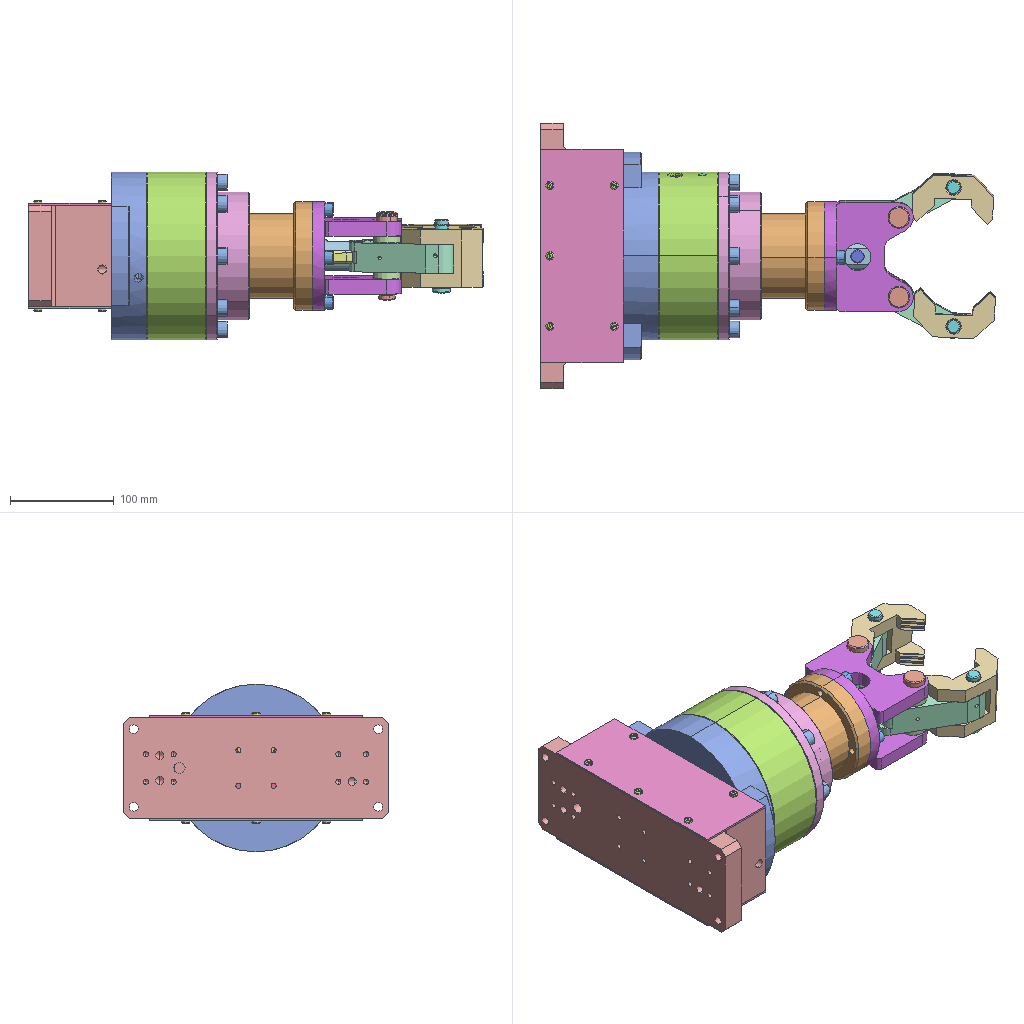Assembly | SolidWorks | 43 different items | 84 placed | box 439 x 256 x 162 mm
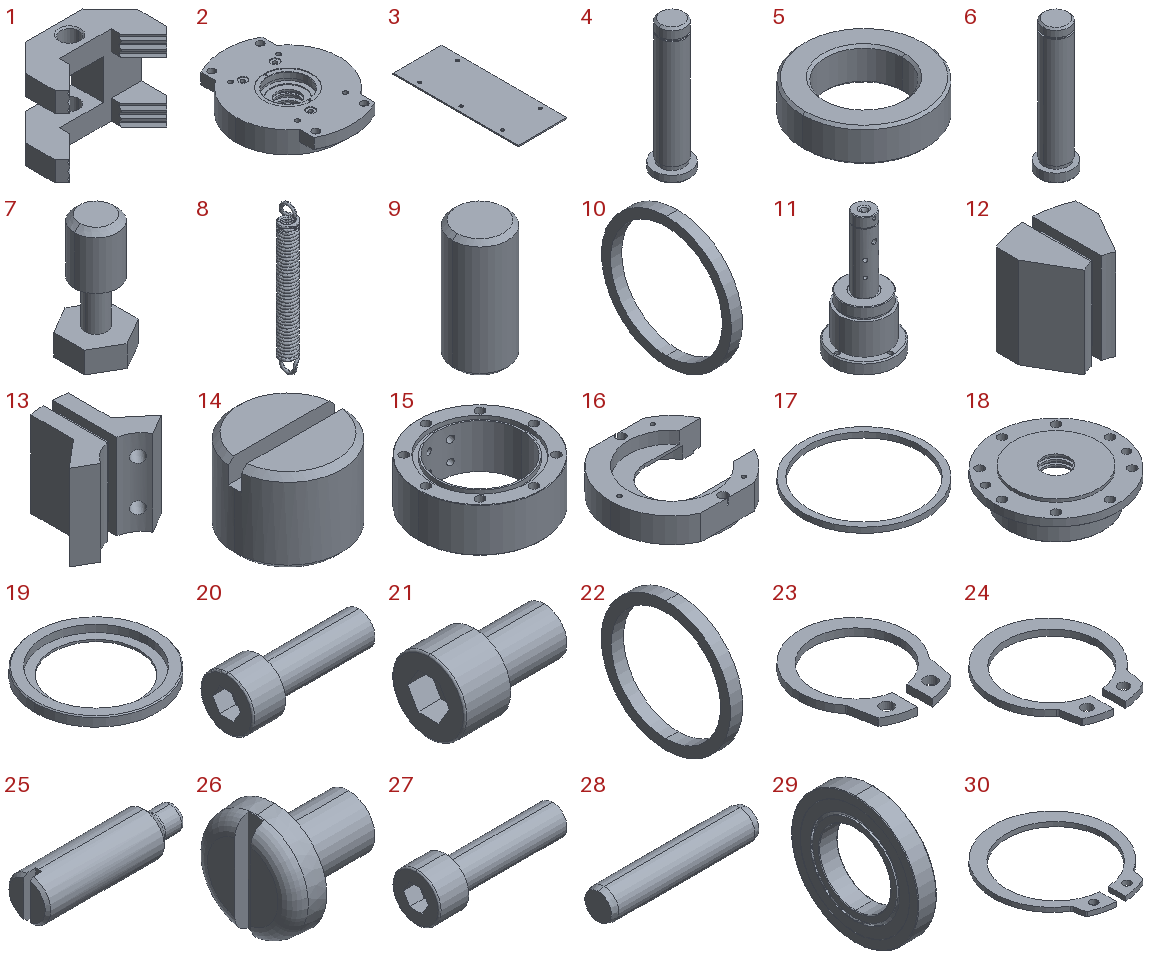Parts list (item | quantity | size | volume | features):
1 | x2 | 78 x 44.997 x 56 mm | 64045 mm3 | features ICE 3, MirrorPattern 2, Chamfer 1, Extrusion 1
2 | x1 | 162 x 200 x 38 mm | 697983 mm3 | features ICE 13, HoleWzd 9, Chamfer 2, 3DProfileFeature 1, CirPattern 1, Extrusion 1, MirrorPattern 1
3 | x2 | 80 x 206 x 2 mm | 32764 mm3 | features Extrusion 1, HoleWzd 1
4 | x2 | 18 x 18 x 66 mm | 9140 mm3 | features ICE 4, Chamfer 1, Extrusion 1
5 | x2 | 26 x 26 x 7 mm | 2241 mm3 | features Chamfer 1, Extrusion 1
6 | x2 | 21 x 21 x 82 mm | 17223 mm3 | features ICE 4, Chamfer 1, Extrusion 1
7 | x1 | 5 x 5.774 x 11 mm | 117.26 mm3 | features ICE 2, Chamfer 1, Extrusion 1
8 | x1 | 5.989 x 6.003 x 53 mm | 518.141 mm3 | features RefCurve 2, CompositeCurve 1, Helix 1, Sweep 1
9 | x1 | 13 x 13 x 28 mm | 3662 mm3 | features 3DProfileFeature 1, Chamfer 1, Extrusion 1, HoleWzd 1
10 | x4 | 3.5 x 40.6 x 40.6 mm | 1164 mm3 | features Extrusion 1
11 | x1 | 105 x 105 x 207 mm | 339830 mm3 | features ICE 8, HoleWzd 5, 3DProfileFeature 4, RevCut 3, Chamfer 2, CirPattern 1, Extrusion 1
12 | x1 | 44 x 39.776 x 50 mm | 60767 mm3 | features 3DProfileFeature 2, HoleWzd 2, Extrusion 1, ICE 1
13 | x1 | 53.823 x 46.181 x 50 mm | 52873 mm3 | features 3DProfileFeature 2, HoleWzd 2, Extrusion 1, ICE 1
14 | x1 | 9.73 x 9.73 x 7.5 mm | 527.297 mm3 | features Chamfer 1, Extrusion 1, ICE 1
15 | x1 | 162 x 162 x 58 mm | 564661 mm3 | features HoleWzd 5, 3DProfileFeature 4, Chamfer 2, ICE 2, CirPattern 1, Extrusion 1, MirrorPattern 1
16 | x1 | 77.837 x 73.95 x 18 mm | 34057 mm3 | features ICE 5, 3DProfileFeature 2, HoleWzd 2, CirPattern 1, Extrusion 1
17 | x2 | 127 x 127 x 5.5 mm | 13534 mm3 | features Extrusion 1
18 | x1 | 162 x 162 x 45 mm | 267421 mm3 | features ICE 12, Chamfer 2, HoleWzd 2, CirPattern 1, Extrusion 1
19 | x1 | 120 x 120 x 9 mm | 34518 mm3 | features Chamfer 1, CirPattern 1, Extrusion 1, HoleWzd 1, ICE 1
20 | x4 | 33 x 13 x 13 mm | 2188 mm3 | features BlendCut 1, Cut 1, Fillet 1, LPattern 1, RevCut 1, Revolution 1
21 | x4 | 26 x 16 x 16 mm | 2981 mm3 | features BlendCut 1, Cut 1, Fillet 1, LPattern 1, RevCut 1, Revolution 1
22 | x2 | 6.2 x 65 x 65 mm | 5843 mm3 | features Extrusion 1
23 | x2 | 14.7 x 17.116 x 1 mm | 75.123 mm3 | features Extrusion 1
24 | x2 | 18.2 x 20.685 x 1 mm | 106.213 mm3 | features Extrusion 1
25 | x1 | 14 x 4 x 4 mm | 151.43 mm3 | features Cut 1, Fillet 1, Revolution 1
26 | x10 | 8.4 x 8 x 8 mm | 170.552 mm3 | features Fillet 2, ICE 1, LPattern 1, RevCut 1, Revolution 1
27 | x2 | 38 x 13 x 13 mm | 2439 mm3 | features BlendCut 1, Cut 1, Fillet 1, LPattern 1, RevCut 1, Revolution 1
28 | x2 | 40 x 8 x 8 mm | 1994 mm3 | features Revolution 1
29 | x1 | 9 x 62 x 62 mm | 14273 mm3 | features Revolution 5, CirPattern 2, RefAxis 1, RevCut 1
30 | x1 | 39 x 42.278 x 1.5 mm | 631.207 mm3 | features Extrusion 1
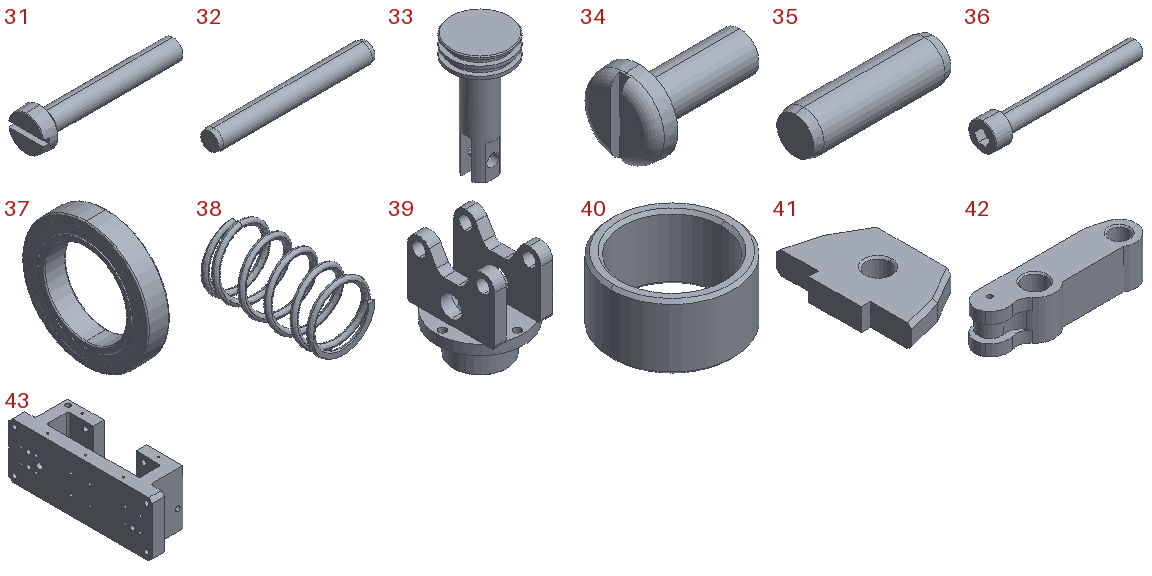31 | x2 | 22 x 5.5 x 5.5 mm | 181.48 mm3 | features Cut 1, LPattern 1, RevCut 1, Revolution 1
32 | x2 | 80 x 10 x 10 mm | 6251 mm3 | features Revolution 1
33 | x1 | 65 x 65 x 132 mm | 129865 mm3 | features ICE 9, Chamfer 2, 3DProfileFeature 1, Extrusion 1, Fillet 1, HoleWzd 1
34 | x2 | 19.6 x 12 x 12 mm | 779.516 mm3 | features Fillet 2, ICE 1, LPattern 1, RevCut 1, Revolution 1
35 | x2 | 20 x 6 x 6 mm | 558.473 mm3 | features Revolution 1
36 | x8 | 90 x 16 x 16 mm | 8007 mm3 | features BlendCut 1, Cut 1, Fillet 1, LPattern 1, RevCut 1, Revolution 1
37 | x1 | 20 x 115 x 115 mm | 89523 mm3 | features Revolution 5, CirPattern 2, RefAxis 1, RevCut 1
38 | x1 | 52.5 x 90 x 52.5 mm | 16226 mm3 | features Sweep 3, ICE 1
39 | x1 | 105 x 105 x 121 mm | 288866 mm3 | features ICE 4, Chamfer 1, CirPattern 1, Extrusion 1, Fillet 1, HoleWzd 1, MirrorPattern 1
40 | x1 | 40 x 40 x 21 mm | 9274 mm3 | features Chamfer 1, Extrusion 1
41 | x1 | 41 x 72 x 12 mm | 25554 mm3 | features Chamfer 2, Extrusion 1
42 | x2 | 109.566 x 29 x 28 mm | 60118 mm3 | features ICE 3, MirrorPattern 2, 3DProfileFeature 1, Chamfer 1, Extrusion 1, HoleWzd 1
43 | x1 | 80 x 256 x 98 mm | 906653 mm3 | features HoleWzd 16, MirrorPattern 3, 3DProfileFeature 2, Chamfer 1, CirPattern 1, Extrusion 1, Fillet 1, ICE 1
Mates (type | each side: item.copy, entity, surface, feature):
Coincident | 43.1 face plane Boss-Extrude2 | 2.1 face plane Boss-Extrude1
Concentric | 43.1 face cylinder M10 Tapped Hole2 | 2.1 face cylinder Mirror1
Concentric | 43.1 face cylinder M10 Tapped Hole2 | 2.1 face cylinder CBORE for M1.6 Hex Head Bolt2
Coincident | 2.1 face plane Boss-Extrude2 | 15.1 face plane Boss-Extrude1
Concentric | 2.1 face cylinder M10 Tapped Hole2 | 15.1 face cylinder Ø5.0mm Blind Dowel Hole1
Concentric | 2.1 face cylinder CirPattern1 | 15.1 face cylinder CirPattern1
Coincident | 15.1 face plane Boss-Extrude1 | 18.1 face plane Boss-Extrude1
Concentric | 15.1 face cylinder Ø5.0mm Blind Dowel Hole1 | 18.1 face cylinder CirPattern1
Concentric | 15.1 face cylinder CirPattern1 | 18.1 face cylinder CirPattern1
Parallel | 18.1 face plane Cut-Extrude6 | 19.1 face plane Boss-Extrude1
Coincident | 18.1 face plane Boss-Extrude3 | 19.1 face plane Boss-Extrude1
Concentric | 18.1 edge | 19.1 edge
Parallel | 19.1 plane | assembly plane
Concentric | 15.1 face cylinder Ø8.0mm Blind Dowel Hole1 | 12.1 face cylinder Ø8.0mm Blind Dowel Hole1
Coincident | 18.1 face plane Boss-Extrude2 | 12.1 face plane Boss-Extrude1
Concentric | 15.1 face cylinder Ø8.0mm Blind Dowel Hole2 | 12.1 face cylinder Ø8.0mm Blind Dowel Hole1
Concentric | 2.1 face cylinder Cut-Extrude11 | 11.1 face cone Cut-Revolve2
Parallel | 13.1 plane | assembly plane
Concentric | 11.1 face cylinder Ø6.0mm Blind Dowel Hole1 | 13.1 face cylinder Ø6.0mm Blind Dowel Hole2
Concentric | 11.1 face cylinder Ø6.0mm Blind Dowel Hole1 | 13.1 face cylinder Ø6.0mm Blind Dowel Hole1
Coincident | 18.1 face plane Boss-Extrude2 | 13.1 face plane Boss-Extrude1
Concentric | 11.1 face cylinder Cut-Revolve2 | 16.1 face cylinder Cut-Extrude5
Parallel | 43.1 face plane Boss-Extrude2 | 16.1 face plane Cut-Extrude1
Coincident | 2.1 face plane Cut-Extrude1 | 16.1 face plane Boss-Extrude2
Concentric | 11.1 edge | 33.1 edge
Concentric | 33.1 face cylinder Cut-Extrude3 | 41.1 face cylinder Boss-Extrude1
Coincident | 33.1 face plane Cut-Extrude1 | 41.1 face plane Boss-Extrude1
Coincident | 11.1 face plane Boss-Extrude1 | 39.1 face plane Boss-Extrude2
Concentric | 11.1 face cylinder M8 Tapped Hole1 | 39.1 face cylinder CirPattern1
Concentric | 11.1 face cylinder CirPattern1 | 39.1 face cylinder Ø5.0mm Blind Dowel Hole1
LimitDistanceDim | 33.1 face plane Boss-Extrude5 | 11.1 face plane Cut-Extrude2
Parallel | 33.1 face plane Cut-Extrude1 | 41.1 face plane Boss-Extrude1
Concentric | 39.1 face cylinder Mirror1 | 42.1 face cylinder Boss-Extrude1
Concentric | 39.1 face cylinder Mirror1 | 42.2 face cylinder Boss-Extrude1
Width | 39.1 face plane Boss-Extrude3 | 39.1 face plane Mirror1 | 42.1 face plane Mirror1 | 42.1 face plane Boss-Extrude2
Concentric | 39.1 face cylinder Boss-Extrude3 | 6.1 face cylinder Boss-Extrude3
Coincident | 39.1 face plane Mirror1 | 6.1 face plane Boss-Extrude1
Width | 39.1 face plane Mirror1 | 39.1 face plane Boss-Extrude3 | 42.2 face plane Mirror1 | 42.2 face plane Boss-Extrude2
Concentric | 39.1 face cylinder Mirror1 | 6.2 face cylinder Boss-Extrude3
Coincident | 39.1 face plane Mirror1 | 6.2 edge
Parallel | 41.1 face plane Boss-Extrude1 | 39.1 face plane Boss-Extrude3
Concentric | 33.1 face cylinder Cut-Extrude3 | 9.1 face cylinder Boss-Extrude1
Width | 9.1 face plane Boss-Extrude1 | 9.1 face plane Boss-Extrude1 | 33.1 face plane Cut-Extrude2 | 33.1 face plane Cut-Extrude2
Concentric | 33.1 face cylinder M4 Tapped Hole1 | 9.1 face cylinder Ø2.5mm Blind Dowel Hole1
Concentric | 6.2 face cylinder Boss-Extrude3 | 5.1 face cylinder Boss-Extrude1
Coincident | 42.2 face plane Boss-Extrude2 | 5.1 face plane Boss-Extrude1
Concentric | 6.2 face cylinder Boss-Extrude3 | 5.2 face cylinder Boss-Extrude1
Coincident | 39.1 face plane Mirror1 | 5.2 face plane Boss-Extrude1
Concentric | 43.1 face cylinder M4 Tapped Hole1 | 3.1 face cylinder Ø5.0mm Blind Dowel Hole1 | 2 times
Coincident | 43.1 face plane Boss-Extrude2 | 3.1 face plane Boss-Extrude1
Concentric | 43.1 face cylinder Mirror1 | 3.2 face cylinder Ø5.0mm Blind Dowel Hole1 | 2 times
Coincident | 43.1 face plane Boss-Extrude2 | 3.2 face plane Boss-Extrude1
Concentric | 42.2 face cylinder Boss-Extrude1 | 1.1 face cylinder Boss-Extrude1
Width | 1.1 face plane Boss-Extrude1 | 1.1 face plane Boss-Extrude1 | 42.2 face plane Boss-Extrude2 | 42.2 face plane Mirror1
Concentric | 4.1 face cylinder Boss-Extrude3 | 1.1 face cylinder Boss-Extrude1
Coincident | 1.1 face plane Boss-Extrude1 | 4.1 face plane Boss-Extrude5
Concentric | 42.1 face cylinder Boss-Extrude1 | 1.2 face cylinder Boss-Extrude1
Width | 1.2 face plane Boss-Extrude1 | 1.2 face plane Boss-Extrude1 | 42.1 face plane Boss-Extrude2 | 42.1 face plane Mirror1
Concentric | 1.2 face cylinder Boss-Extrude1 | 4.2 face cylinder Boss-Extrude3
Coincident | 1.2 face plane Boss-Extrude1 | 4.2 face plane Boss-Extrude5
Tangent | 41.1 face plane Boss-Extrude1 | 42.2 face cylinder Boss-Extrude1
Tangent | 41.1 face plane Boss-Extrude1 | 42.1 face cylinder Boss-Extrude1
Concentric | 11.1 face cylinder Cut-Revolve1 | 17.1 face cylinder Boss-Extrude1
Coincident | 2.1 face plane Boss-Extrude2 | 17.1 face plane Boss-Extrude1
Concentric | 11.1 face cylinder Cut-Revolve1 | 17.2 face cylinder Boss-Extrude1
Coincident | 18.1 face plane Boss-Extrude1 | 17.2 edge
Concentric | 11.1 face cylinder Cut-Extrude1 | 22.1 face cylinder Boss-Extrude1
Concentric | 11.1 face cylinder Cut-Extrude1 | 22.2 edge
Coincident | 33.1 face plane Boss-Extrude5 | 22.2 face plane Boss-Extrude1
Coincident | 33.1 face plane Boss-Extrude3 | 22.1 face plane Boss-Extrude1
Concentric | 11.1 face cylinder Cut-Revolve1 | 10.1 face cylinder Boss-Extrude1
Coincident | 18.1 face plane Cut-Extrude4 | 10.1 face plane Boss-Extrude1
Concentric | 11.1 face cylinder Cut-Revolve1 | 10.2 face cylinder Boss-Extrude1
Coincident | 18.1 face plane Cut-Extrude2 | 10.2 face plane Boss-Extrude1
Concentric | 11.1 face cylinder Cut-Revolve1 | 10.3 face cylinder Boss-Extrude1
Coincident | 2.1 face plane Cut-Extrude3 | 10.3 face plane Boss-Extrude1
Concentric | 11.1 face cylinder Cut-Revolve1 | 10.4 face cylinder Boss-Extrude1
Coincident | 2.1 face plane Cut-Extrude7 | 10.4 face plane Boss-Extrude1
Concentric | 18.1 face cylinder CirPattern1 | 36.1 face cylinder Base-Revolve
Coincident | 18.1 face plane Boss-Extrude1 | 36.1 face plane Base-Revolve
Concentric | 18.1 face cylinder CirPattern1 | 36.2 face cylinder Base-Revolve
Coincident | 18.1 face plane Boss-Extrude1 | 36.2 face plane Base-Revolve
Concentric | 18.1 face cylinder CirPattern1 | 36.3 face cylinder Base-Revolve
Coincident | 18.1 face plane Boss-Extrude1 | 36.3 face plane Base-Revolve
Concentric | 18.1 face cylinder Ø1.0mm Blind Dowel Hole1 | 36.4 face cylinder Base-Revolve
Coincident | 18.1 face plane Boss-Extrude1 | 36.4 edge
Concentric | 18.1 face cylinder CirPattern1 | 36.5 face cylinder Base-Revolve
Coincident | 18.1 face plane Boss-Extrude1 | 36.5 face plane Base-Revolve
Concentric | 18.1 face cylinder CirPattern1 | 36.6 face cylinder Base-Revolve
Coincident | 18.1 face plane Boss-Extrude1 | 36.6 face plane Base-Revolve
Concentric | 18.1 face cylinder CirPattern1 | 36.7 face cylinder Base-Revolve
Coincident | 18.1 face plane Boss-Extrude1 | 36.7 face plane Base-Revolve
Concentric | 18.1 face cylinder CirPattern1 | 36.8 face cylinder Base-Revolve
Coincident | 18.1 face plane Boss-Extrude1 | 36.8 edge
Concentric | 3.1 face cylinder Ø5.0mm Blind Dowel Hole1 | 26.1 face cylinder Base-Revolve
Coincident | 3.1 face plane Boss-Extrude1 | 26.1 face plane Base-Revolve
Concentric | 3.1 face cylinder Ø5.0mm Blind Dowel Hole1 | 26.2 face cylinder Base-Revolve
Coincident | 3.1 face plane Boss-Extrude1 | 26.2 face plane Base-Revolve
Concentric | 3.1 face cylinder Ø5.0mm Blind Dowel Hole1 | 26.3 face cylinder Base-Revolve
Coincident | 3.1 face plane Boss-Extrude1 | 26.3 face plane Base-Revolve
Concentric | 15.1 edge | 27.1 face cylinder Base-Revolve
Coincident | 15.1 face plane CBORE for M1.6 Hex Head Bolt1 | 27.1 face plane Base-Revolve
Concentric | 15.1 face cylinder Ø8.0mm Blind Dowel Hole2 | 28.1 face cylinder Base-Revolve
Tangent | 15.1 face cylinder Boss-Extrude1 | 28.1 face plane Base-Revolve
Concentric | 15.1 face cylinder CBORE for M6 Hex Head Bolt1 | 27.2 face cylinder Base-Revolve
Coincident | 15.1 face plane CBORE for M6 Hex Head Bolt1 | 27.2 face plane Base-Revolve
Concentric | 15.1 face cylinder Ø8.0mm Blind Dowel Hole1 | 28.2 face cylinder Base-Revolve
Tangent | 15.1 face cylinder Boss-Extrude1 | 28.2 face plane Base-Revolve
Concentric | 13.1 face cylinder Ø6.0mm Blind Dowel Hole2 | 34.1 face cylinder Base-Revolve
Concentric | 13.1 face cylinder Ø6.0mm Blind Dowel Hole2 | 34.2 face cylinder Base-Revolve
Coincident | 13.1 face plane Boss-Extrude1 | 34.1 face plane Base-Revolve
Coincident | 13.1 face plane Boss-Extrude1 | 34.2 face plane Base-Revolve
Concentric | 13.1 face cylinder Ø6.0mm Blind Dowel Hole1 | 35.1 face cylinder Base-Revolve
Coincident | 13.1 face plane Boss-Extrude1 | 35.1 face plane Base-Revolve
Concentric | 13.1 face cylinder Ø6.0mm Blind Dowel Hole1 | 35.2 face cylinder Base-Revolve
Coincident | 13.1 face plane Boss-Extrude1 | 35.2 face plane Base-Revolve
Concentric | 11.1 face cylinder Cut-Revolve1 | 37.1 face cylinder Revolve1
Coincident | 18.1 face plane Cut-Extrude7 | 37.1 face plane Revolve1
Concentric | 11.1 face cylinder Cut-Revolve2 | 29.1 face cylinder Revolve1
Coincident | 2.1 face plane Cut-Extrude10 | 29.1 face plane Revolve1
Concentric | 11.1 face cylinder Cut-Revolve2 | 30.1 face cylinder Base-Extrude
Coincident | 11.1 face plane Cut-Extrude6 | 30.1 face plane Base-Extrude
Concentric | 6.1 face cylinder Boss-Extrude4 | 24.1 face cylinder Base-Extrude
Coincident | 6.1 face plane Boss-Extrude5 | 24.1 face plane Base-Extrude
Concentric | 6.2 face cylinder Boss-Extrude4 | 24.2 face cylinder Base-Extrude
Coincident | 6.2 face plane Boss-Extrude5 | 24.2 face plane Base-Extrude
Concentric | 4.2 face cylinder Boss-Extrude2 | 23.1 face cylinder Base-Extrude
Coincident | 4.2 face plane Boss-Extrude1 | 23.1 face plane Base-Extrude
Concentric | 4.1 face cylinder Boss-Extrude2 | 23.2 face cylinder Base-Extrude
Coincident | 4.1 face plane Boss-Extrude1 | 23.2 face plane Base-Extrude
Concentric | 39.1 face cylinder CirPattern1 | 20.1 face cylinder Base-Revolve
Coincident | 39.1 face plane Boss-Extrude2 | 20.1 face plane Base-Revolve
Concentric | 39.1 face cylinder CirPattern1 | 20.2 face cylinder Base-Revolve
Coincident | 39.1 face plane Boss-Extrude2 | 20.2 face plane Base-Revolve
Concentric | 39.1 face cylinder CirPattern1 | 20.3 face cylinder Base-Revolve
Coincident | 39.1 face plane Boss-Extrude2 | 20.3 face plane Base-Revolve
Concentric | 39.1 face cylinder Ø5.0mm Blind Dowel Hole1 | 20.4 face cylinder Base-Revolve
Coincident | 39.1 face plane Boss-Extrude2 | 20.4 face plane Base-Revolve
Concentric | 2.1 face cylinder Mirror1 | 21.1 face cylinder Base-Revolve
Coincident | 2.1 face plane Mirror1 | 21.1 face plane Base-Revolve
Concentric | 33.1 face cylinder M4 Tapped Hole1 | 25.1 face cylinder Base-Revolve
Coincident | 33.1 face plane Boss-Extrude7 | 25.1 face plane Base-Revolve
Concentric | 16.1 face cylinder CBORE for M3 Hex Head Bolt3 | 31.1 face cylinder Base-Revolve
Coincident | 16.1 face plane CBORE for M3 Hex Head Bolt3 | 31.1 face plane Base-Revolve
Concentric | 18.1 face cylinder Ø10.0mm Blind Dowel Hole1 | 32.1 face cylinder Base-Revolve
Coincident | 18.1 face plane Boss-Extrude1 | 32.1 face plane Base-Revolve
Concentric | 18.1 face cylinder Ø10.0mm Blind Dowel Hole1 | 32.2 face cylinder Base-Revolve
Coincident | 18.1 face plane Boss-Extrude1 | 32.2 face plane Base-Revolve